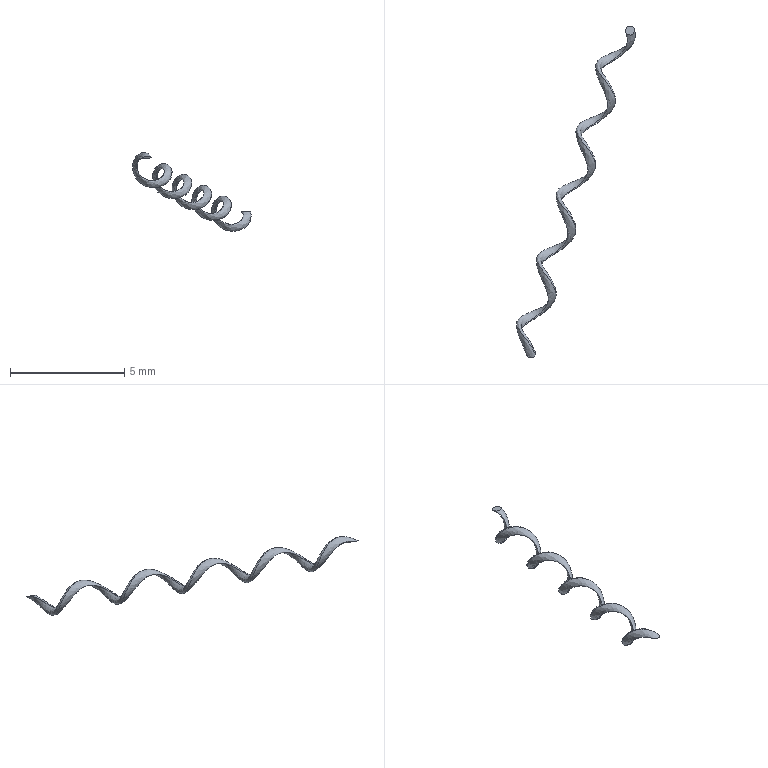Part | SolidWorks | features BaseBody 1 | 1 solid | 4 faces | box 5.217 x 14.553 x 3.46 mm | volume 1.395 mm3 | spline 2 | plane 2